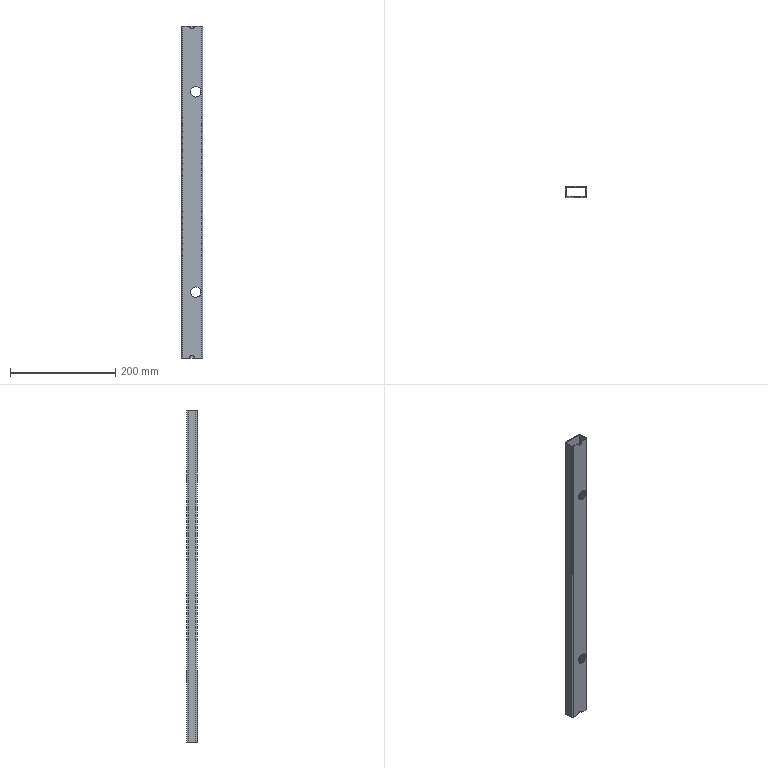Part | STEP file | 5090107 | 1 solid | 24 faces | box 40 x 20 x 630 mm | volume 102888 mm3 | cylinder 14 | plane 10 | commonest cylinder face diameters 2 x4 5 x4 20 x4 10 x2